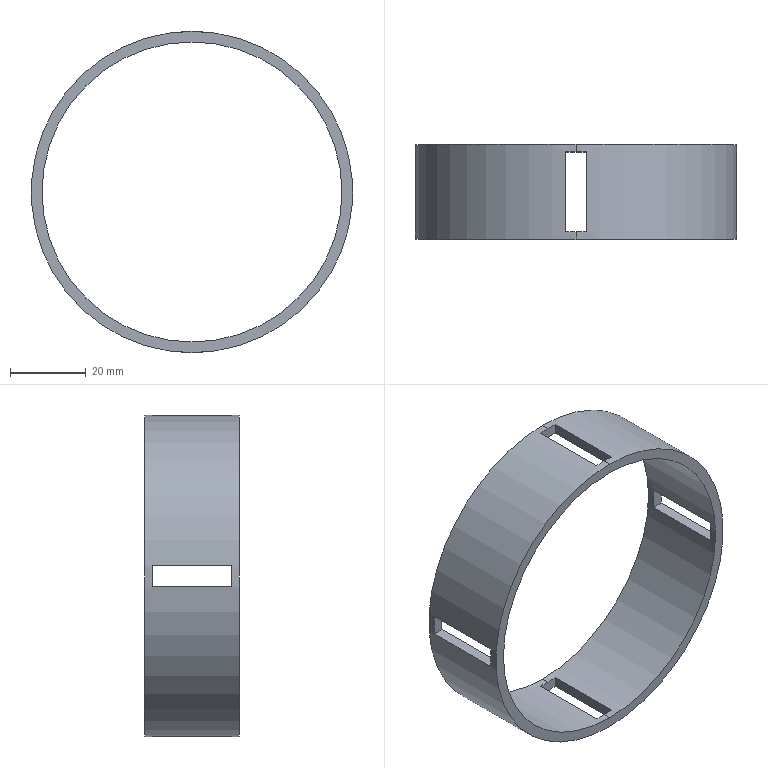Part | SolidWorks | features BaseBody 1 | 1 solid | 22 faces | box 84.688 x 25 x 84.688 mm | volume 16756 mm3 | plane 18 | cylinder 4 | commonest cylinder face diameters 79.062 x2 84.687 x2
STEP:
#1=CARTESIAN_POINT('',(-2132.95,780.069,-1538.093));
#2=VERTEX_POINT('',#1);
#3=CARTESIAN_POINT('',(-2132.95,780.069,-1617.156));
#4=VERTEX_POINT('',#3);
#5=CARTESIAN_POINT('',(-2132.95,780.069,-1577.624));
#6=DIRECTION('',(0.,1.,0.));
#7=DIRECTION('',(0.,0.,1.));
#8=AXIS2_PLACEMENT_3D('',#5,#6,#7);
#9=CIRCLE('',#8,39.531);
#10=EDGE_CURVE('',#2,#4,#9,.T.);
#11=ORIENTED_EDGE('',*,*,#10,.F.);
#12=CARTESIAN_POINT('',(-2132.95,780.069,-1577.624));
#13=DIRECTION('',(0.,1.,0.));
#14=DIRECTION('',(0.,0.,-1.));
#15=AXIS2_PLACEMENT_3D('',#12,#13,#14);
#16=CIRCLE('',#15,39.531);
#17=EDGE_CURVE('',#4,#2,#16,.T.);
#18=ORIENTED_EDGE('',*,*,#17,.F.);
#19=EDGE_LOOP('',(#11,#18));
#20=FACE_BOUND('',#19,.T.);
#21=CARTESIAN_POINT('',(-2132.95,780.069,-1619.968));
#22=VERTEX_POINT('',#21);
#23=CARTESIAN_POINT('',(-2132.95,780.069,-1535.281));
#24=VERTEX_POINT('',#23);
#25=CARTESIAN_POINT('',(-2132.95,780.069,-1577.624));
#26=DIRECTION('',(0.,1.,0.));
#27=DIRECTION('',(0.,0.,-1.));
#28=AXIS2_PLACEMENT_3D('',#25,#26,#27);
#29=CIRCLE('',#28,42.344);
#30=EDGE_CURVE('',#22,#24,#29,.T.);
#31=ORIENTED_EDGE('',*,*,#30,.T.);
#32=CARTESIAN_POINT('',(-2132.95,780.069,-1577.624));
#33=DIRECTION('',(0.,1.,0.));
#34=DIRECTION('',(0.,0.,1.));
#35=AXIS2_PLACEMENT_3D('',#32,#33,#34);
#36=CIRCLE('',#35,42.344);
#37=EDGE_CURVE('',#24,#22,#36,.T.);
#38=ORIENTED_EDGE('',*,*,#37,.T.);
#39=EDGE_LOOP('',(#31,#38));
#40=FACE_OUTER_BOUND('',#39,.T.);
#41=CARTESIAN_POINT('',(-2086.372,780.069,-1531.046));
#42=DIRECTION('',(0.,1.,0.));
#43=DIRECTION('',(1.,0.,0.));
#44=AXIS2_PLACEMENT_3D('',#41,#42,#43);
#45=PLANE('',#44);
#46=ADVANCED_FACE('',(#20,#40),#45,.T.);
#47=CARTESIAN_POINT('',(-2132.95,755.069,-1538.093));
#48=VERTEX_POINT('',#47);
#49=CARTESIAN_POINT('',(-2132.95,755.069,-1617.156));
#50=VERTEX_POINT('',#49);
#51=CARTESIAN_POINT('',(-2132.95,755.069,-1577.624));
#52=DIRECTION('',(0.,-1.,0.));
#53=DIRECTION('',(0.,0.,1.));
#54=AXIS2_PLACEMENT_3D('',#51,#52,#53);
#55=CIRCLE('',#54,39.531);
#56=EDGE_CURVE('',#48,#50,#55,.T.);
#57=ORIENTED_EDGE('',*,*,#56,.F.);
#58=CARTESIAN_POINT('',(-2132.95,755.069,-1577.624));
#59=DIRECTION('',(0.,-1.,0.));
#60=DIRECTION('',(0.,0.,-1.));
#61=AXIS2_PLACEMENT_3D('',#58,#59,#60);
#62=CIRCLE('',#61,39.531);
#63=EDGE_CURVE('',#50,#48,#62,.T.);
#64=ORIENTED_EDGE('',*,*,#63,.F.);
#65=EDGE_LOOP('',(#57,#64));
#66=FACE_BOUND('',#65,.T.);
#67=CARTESIAN_POINT('',(-2132.95,755.069,-1619.968));
#68=VERTEX_POINT('',#67);
#69=CARTESIAN_POINT('',(-2132.95,755.069,-1535.281));
#70=VERTEX_POINT('',#69);
#71=CARTESIAN_POINT('',(-2132.95,755.069,-1577.624));
#72=DIRECTION('',(0.,-1.,0.));
#73=DIRECTION('',(0.,0.,-1.));
#74=AXIS2_PLACEMENT_3D('',#71,#72,#73);
#75=CIRCLE('',#74,42.344);
#76=EDGE_CURVE('',#68,#70,#75,.T.);
#77=ORIENTED_EDGE('',*,*,#76,.T.);
#78=CARTESIAN_POINT('',(-2132.95,755.069,-1577.624));
#79=DIRECTION('',(0.,-1.,0.));
#80=DIRECTION('',(0.,0.,1.));
#81=AXIS2_PLACEMENT_3D('',#78,#79,#80);
#82=CIRCLE('',#81,42.344);
#83=EDGE_CURVE('',#70,#68,#82,.T.);
#84=ORIENTED_EDGE('',*,*,#83,.T.);
#85=EDGE_LOOP('',(#77,#84));
#86=FACE_OUTER_BOUND('',#85,.T.);
#87=CARTESIAN_POINT('',(-2086.372,755.069,-1624.203));
#88=DIRECTION('',(0.,-1.,0.));
#89=DIRECTION('',(0.,0.,-1.));
#90=AXIS2_PLACEMENT_3D('',#87,#88,#89);
#91=PLANE('',#90);
#92=ADVANCED_FACE('',(#66,#86),#91,.T.);
#93=CARTESIAN_POINT('',(-2090.699,757.069,-1574.812));
#94=VERTEX_POINT('',#93);
#95=CARTESIAN_POINT('',(-2090.699,757.069,-1580.437));
#96=VERTEX_POINT('',#95);
#97=CARTESIAN_POINT('',(-2132.95,757.069,-1577.624));
#98=DIRECTION('',(0.,1.,0.));
#99=DIRECTION('',(0.9978,0.,0.06642));
#100=AXIS2_PLACEMENT_3D('',#97,#98,#99);
#101=CIRCLE('',#100,42.344);
#102=EDGE_CURVE('',#94,#96,#101,.T.);
#103=ORIENTED_EDGE('',*,*,#102,.F.);
#104=CARTESIAN_POINT('',(-2090.699,778.069,-1574.812));
#105=VERTEX_POINT('',#104);
#106=CARTESIAN_POINT('',(-2090.699,757.069,-1574.812));
#107=DIRECTION('',(0.,1.,0.));
#108=VECTOR('',#107,1000.);
#109=LINE('',#106,#108);
#110=EDGE_CURVE('',#94,#105,#109,.T.);
#111=ORIENTED_EDGE('',*,*,#110,.T.);
#112=CARTESIAN_POINT('',(-2090.699,778.069,-1580.437));
#113=VERTEX_POINT('',#112);
#114=CARTESIAN_POINT('',(-2132.95,778.069,-1577.624));
#115=DIRECTION('',(0.,-1.,0.));
#116=DIRECTION('',(0.9978,0.,-0.06642));
#117=AXIS2_PLACEMENT_3D('',#114,#115,#116);
#118=CIRCLE('',#117,42.344);
#119=EDGE_CURVE('',#113,#105,#118,.T.);
#120=ORIENTED_EDGE('',*,*,#119,.F.);
#121=CARTESIAN_POINT('',(-2090.699,778.069,-1580.437));
#122=DIRECTION('',(0.,-1.,0.));
#123=VECTOR('',#122,1000.);
#124=LINE('',#121,#123);
#125=EDGE_CURVE('',#113,#96,#124,.T.);
#126=ORIENTED_EDGE('',*,*,#125,.T.);
#127=EDGE_LOOP('',(#103,#111,#120,#126));
#128=FACE_BOUND('',#127,.T.);
#129=CARTESIAN_POINT('',(-2132.95,757.069,-1619.968));
#130=VERTEX_POINT('',#129);
#131=CARTESIAN_POINT('',(-2132.95,755.069,-1619.968));
#132=DIRECTION('',(0.,1.,0.));
#133=VECTOR('',#132,1000.);
#134=LINE('',#131,#133);
#135=EDGE_CURVE('',#68,#130,#134,.T.);
#136=ORIENTED_EDGE('',*,*,#135,.T.);
#137=CARTESIAN_POINT('',(-2130.137,757.069,-1619.875));
#138=VERTEX_POINT('',#137);
#139=CARTESIAN_POINT('',(-2132.95,757.069,-1577.624));
#140=DIRECTION('',(0.,1.,0.));
#141=DIRECTION('',(0.06642,0.,-0.9978));
#142=AXIS2_PLACEMENT_3D('',#139,#140,#141);
#143=CIRCLE('',#142,42.344);
#144=EDGE_CURVE('',#138,#130,#143,.T.);
#145=ORIENTED_EDGE('',*,*,#144,.F.);
#146=CARTESIAN_POINT('',(-2130.137,778.069,-1619.875));
#147=VERTEX_POINT('',#146);
#148=CARTESIAN_POINT('',(-2130.137,757.069,-1619.875));
#149=DIRECTION('',(0.,1.,0.));
#150=VECTOR('',#149,1000.);
#151=LINE('',#148,#150);
#152=EDGE_CURVE('',#138,#147,#151,.T.);
#153=ORIENTED_EDGE('',*,*,#152,.T.);
#154=CARTESIAN_POINT('',(-2132.95,778.069,-1619.968));
#155=VERTEX_POINT('',#154);
#156=CARTESIAN_POINT('',(-2132.95,778.069,-1577.624));
#157=DIRECTION('',(0.,-1.,0.));
#158=DIRECTION('',(0.,0.,-1.));
#159=AXIS2_PLACEMENT_3D('',#156,#157,#158);
#160=CIRCLE('',#159,42.344);
#161=EDGE_CURVE('',#155,#147,#160,.T.);
#162=ORIENTED_EDGE('',*,*,#161,.F.);
#163=CARTESIAN_POINT('',(-2132.95,778.069,-1619.968));
#164=DIRECTION('',(0.,1.,0.));
#165=VECTOR('',#164,1000.);
#166=LINE('',#163,#165);
#167=EDGE_CURVE('',#155,#22,#166,.T.);
#168=ORIENTED_EDGE('',*,*,#167,.T.);
#169=ORIENTED_EDGE('',*,*,#37,.F.);
#170=CARTESIAN_POINT('',(-2132.95,778.069,-1535.281));
#171=VERTEX_POINT('',#170);
#172=CARTESIAN_POINT('',(-2132.95,780.069,-1535.281));
#173=DIRECTION('',(0.,-1.,0.));
#174=VECTOR('',#173,1000.);
#175=LINE('',#172,#174);
#176=EDGE_CURVE('',#24,#171,#175,.T.);
#177=ORIENTED_EDGE('',*,*,#176,.T.);
#178=CARTESIAN_POINT('',(-2130.137,778.069,-1535.374));
#179=VERTEX_POINT('',#178);
#180=CARTESIAN_POINT('',(-2132.95,778.069,-1577.624));
#181=DIRECTION('',(0.,-1.,0.));
#182=DIRECTION('',(0.06642,0.,0.9978));
#183=AXIS2_PLACEMENT_3D('',#180,#181,#182);
#184=CIRCLE('',#183,42.344);
#185=EDGE_CURVE('',#179,#171,#184,.T.);
#186=ORIENTED_EDGE('',*,*,#185,.F.);
#187=CARTESIAN_POINT('',(-2130.137,757.069,-1535.374));
#188=VERTEX_POINT('',#187);
#189=CARTESIAN_POINT('',(-2130.137,778.069,-1535.374));
#190=DIRECTION('',(0.,-1.,0.));
#191=VECTOR('',#190,1000.);
#192=LINE('',#189,#191);
#193=EDGE_CURVE('',#179,#188,#192,.T.);
#194=ORIENTED_EDGE('',*,*,#193,.T.);
#195=CARTESIAN_POINT('',(-2132.95,757.069,-1535.281));
#196=VERTEX_POINT('',#195);
#197=CARTESIAN_POINT('',(-2132.95,757.069,-1577.624));
#198=DIRECTION('',(0.,1.,0.));
#199=DIRECTION('',(0.,0.,1.));
#200=AXIS2_PLACEMENT_3D('',#197,#198,#199);
#201=CIRCLE('',#200,42.344);
#202=EDGE_CURVE('',#196,#188,#201,.T.);
#203=ORIENTED_EDGE('',*,*,#202,.F.);
#204=CARTESIAN_POINT('',(-2132.95,757.069,-1535.281));
#205=DIRECTION('',(0.,-1.,0.));
#206=VECTOR('',#205,1000.);
#207=LINE('',#204,#206);
#208=EDGE_CURVE('',#196,#70,#207,.T.);
#209=ORIENTED_EDGE('',*,*,#208,.T.);
#210=ORIENTED_EDGE('',*,*,#76,.F.);
#211=EDGE_LOOP('',(#136,#145,#153,#162,#168,#169,#177,#186,#194,#203,#209,#210));
#212=FACE_OUTER_BOUND('',#211,.T.);
#213=CARTESIAN_POINT('',(-2132.95,753.819,-1577.624));
#214=DIRECTION('',(0.,-1.,0.));
#215=DIRECTION('',(-0.08716,0.,-0.9962));
#216=AXIS2_PLACEMENT_3D('',#213,#214,#215);
#217=CYLINDRICAL_SURFACE('',#216,42.344);
#218=ADVANCED_FACE('',(#128,#212),#217,.T.);
#219=CARTESIAN_POINT('',(-2093.519,757.069,-1574.812));
#220=VERTEX_POINT('',#219);
#221=CARTESIAN_POINT('',(-2093.519,757.069,-1580.437));
#222=VERTEX_POINT('',#221);
#223=CARTESIAN_POINT('',(-2132.95,757.069,-1577.624));
#224=DIRECTION('',(0.,1.,0.));
#225=DIRECTION('',(0.9975,0.,0.07115));
#226=AXIS2_PLACEMENT_3D('',#223,#224,#225);
#227=CIRCLE('',#226,39.531);
#228=EDGE_CURVE('',#220,#222,#227,.T.);
#229=ORIENTED_EDGE('',*,*,#228,.T.);
#230=CARTESIAN_POINT('',(-2093.519,778.069,-1580.437));
#231=VERTEX_POINT('',#230);
#232=CARTESIAN_POINT('',(-2093.519,757.069,-1580.437));
#233=DIRECTION('',(0.,1.,0.));
#234=VECTOR('',#233,1000.);
#235=LINE('',#232,#234);
#236=EDGE_CURVE('',#222,#231,#235,.T.);
#237=ORIENTED_EDGE('',*,*,#236,.T.);
#238=CARTESIAN_POINT('',(-2093.519,778.069,-1574.812));
#239=VERTEX_POINT('',#238);
#240=CARTESIAN_POINT('',(-2132.95,778.069,-1577.624));
#241=DIRECTION('',(0.,-1.,0.));
#242=DIRECTION('',(0.9975,0.,-0.07115));
#243=AXIS2_PLACEMENT_3D('',#240,#241,#242);
#244=CIRCLE('',#243,39.531);
#245=EDGE_CURVE('',#231,#239,#244,.T.);
#246=ORIENTED_EDGE('',*,*,#245,.T.);
#247=CARTESIAN_POINT('',(-2093.519,778.069,-1574.812));
#248=DIRECTION('',(0.,-1.,0.));
#249=VECTOR('',#248,1000.);
#250=LINE('',#247,#249);
#251=EDGE_CURVE('',#239,#220,#250,.T.);
#252=ORIENTED_EDGE('',*,*,#251,.T.);
#253=EDGE_LOOP('',(#229,#237,#246,#252));
#254=FACE_BOUND('',#253,.T.);
#255=CARTESIAN_POINT('',(-2132.95,778.069,-1617.156));
#256=VERTEX_POINT('',#255);
#257=CARTESIAN_POINT('',(-2132.95,780.069,-1617.156));
#258=DIRECTION('',(0.,-1.,0.));
#259=VECTOR('',#258,1000.);
#260=LINE('',#257,#259);
#261=EDGE_CURVE('',#4,#256,#260,.T.);
#262=ORIENTED_EDGE('',*,*,#261,.T.);
#263=CARTESIAN_POINT('',(-2130.137,778.069,-1617.055));
#264=VERTEX_POINT('',#263);
#265=CARTESIAN_POINT('',(-2132.95,778.069,-1577.624));
#266=DIRECTION('',(0.,-1.,0.));
#267=DIRECTION('',(0.,0.,-1.));
#268=AXIS2_PLACEMENT_3D('',#265,#266,#267);
#269=CIRCLE('',#268,39.531);
#270=EDGE_CURVE('',#256,#264,#269,.T.);
#271=ORIENTED_EDGE('',*,*,#270,.T.);
#272=CARTESIAN_POINT('',(-2130.137,757.069,-1617.055));
#273=VERTEX_POINT('',#272);
#274=CARTESIAN_POINT('',(-2130.137,778.069,-1617.055));
#275=DIRECTION('',(0.,-1.,0.));
#276=VECTOR('',#275,1000.);
#277=LINE('',#274,#276);
#278=EDGE_CURVE('',#264,#273,#277,.T.);
#279=ORIENTED_EDGE('',*,*,#278,.T.);
#280=CARTESIAN_POINT('',(-2132.95,757.069,-1617.156));
#281=VERTEX_POINT('',#280);
#282=CARTESIAN_POINT('',(-2132.95,757.069,-1577.624));
#283=DIRECTION('',(0.,1.,0.));
#284=DIRECTION('',(0.07115,0.,-0.9975));
#285=AXIS2_PLACEMENT_3D('',#282,#283,#284);
#286=CIRCLE('',#285,39.531);
#287=EDGE_CURVE('',#273,#281,#286,.T.);
#288=ORIENTED_EDGE('',*,*,#287,.T.);
#289=CARTESIAN_POINT('',(-2132.95,757.069,-1617.156));
#290=DIRECTION('',(0.,-1.,0.));
#291=VECTOR('',#290,1000.);
#292=LINE('',#289,#291);
#293=EDGE_CURVE('',#281,#50,#292,.T.);
#294=ORIENTED_EDGE('',*,*,#293,.T.);
#295=ORIENTED_EDGE('',*,*,#63,.T.);
#296=CARTESIAN_POINT('',(-2132.95,757.069,-1538.093));
#297=VERTEX_POINT('',#296);
#298=CARTESIAN_POINT('',(-2132.95,755.069,-1538.093));
#299=DIRECTION('',(0.,1.,0.));
#300=VECTOR('',#299,1000.);
#301=LINE('',#298,#300);
#302=EDGE_CURVE('',#48,#297,#301,.T.);
#303=ORIENTED_EDGE('',*,*,#302,.T.);
#304=CARTESIAN_POINT('',(-2130.137,757.069,-1538.193));
#305=VERTEX_POINT('',#304);
#306=CARTESIAN_POINT('',(-2132.95,757.069,-1577.624));
#307=DIRECTION('',(0.,1.,0.));
#308=DIRECTION('',(0.,0.,1.));
#309=AXIS2_PLACEMENT_3D('',#306,#307,#308);
#310=CIRCLE('',#309,39.531);
#311=EDGE_CURVE('',#297,#305,#310,.T.);
#312=ORIENTED_EDGE('',*,*,#311,.T.);
#313=CARTESIAN_POINT('',(-2130.137,778.069,-1538.193));
#314=VERTEX_POINT('',#313);
#315=CARTESIAN_POINT('',(-2130.137,757.069,-1538.193));
#316=DIRECTION('',(0.,1.,0.));
#317=VECTOR('',#316,1000.);
#318=LINE('',#315,#317);
#319=EDGE_CURVE('',#305,#314,#318,.T.);
#320=ORIENTED_EDGE('',*,*,#319,.T.);
#321=CARTESIAN_POINT('',(-2132.95,778.069,-1538.093));
#322=VERTEX_POINT('',#321);
#323=CARTESIAN_POINT('',(-2132.95,778.069,-1577.624));
#324=DIRECTION('',(0.,-1.,0.));
#325=DIRECTION('',(0.07115,0.,0.9975));
#326=AXIS2_PLACEMENT_3D('',#323,#324,#325);
#327=CIRCLE('',#326,39.531);
#328=EDGE_CURVE('',#314,#322,#327,.T.);
#329=ORIENTED_EDGE('',*,*,#328,.T.);
#330=CARTESIAN_POINT('',(-2132.95,778.069,-1538.093));
#331=DIRECTION('',(0.,1.,0.));
#332=VECTOR('',#331,1000.);
#333=LINE('',#330,#332);
#334=EDGE_CURVE('',#322,#2,#333,.T.);
#335=ORIENTED_EDGE('',*,*,#334,.T.);
#336=ORIENTED_EDGE('',*,*,#10,.T.);
#337=EDGE_LOOP('',(#262,#271,#279,#288,#294,#295,#303,#312,#320,#329,#335,#336));
#338=FACE_OUTER_BOUND('',#337,.T.);
#339=CARTESIAN_POINT('',(-2132.95,781.319,-1577.624));
#340=DIRECTION('',(0.,-1.,0.));
#341=DIRECTION('',(-0.08716,0.,-0.9962));
#342=AXIS2_PLACEMENT_3D('',#339,#340,#341);
#343=CYLINDRICAL_SURFACE('',#342,39.531);
#344=ADVANCED_FACE('',(#254,#338),#343,.F.);
#345=CARTESIAN_POINT('',(-2135.762,757.069,-1617.055));
#346=VERTEX_POINT('',#345);
#347=CARTESIAN_POINT('',(-2135.762,778.069,-1617.055));
#348=VERTEX_POINT('',#347);
#349=CARTESIAN_POINT('',(-2135.762,757.069,-1617.055));
#350=DIRECTION('',(0.,1.,0.));
#351=VECTOR('',#350,1000.);
#352=LINE('',#349,#351);
#353=EDGE_CURVE('',#346,#348,#352,.T.);
#354=ORIENTED_EDGE('',*,*,#353,.F.);
#355=CARTESIAN_POINT('',(-2135.762,757.069,-1619.875));
#356=VERTEX_POINT('',#355);
#357=CARTESIAN_POINT('',(-2135.762,757.069,-1617.055));
#358=DIRECTION('',(0.,0.,-1.));
#359=VECTOR('',#358,1000.);
#360=LINE('',#357,#359);
#361=EDGE_CURVE('',#346,#356,#360,.T.);
#362=ORIENTED_EDGE('',*,*,#361,.T.);
#363=CARTESIAN_POINT('',(-2135.762,778.069,-1619.875));
#364=VERTEX_POINT('',#363);
#365=CARTESIAN_POINT('',(-2135.762,778.069,-1619.875));
#366=DIRECTION('',(0.,-1.,0.));
#367=VECTOR('',#366,1000.);
#368=LINE('',#365,#367);
#369=EDGE_CURVE('',#364,#356,#368,.T.);
#370=ORIENTED_EDGE('',*,*,#369,.F.);
#371=CARTESIAN_POINT('',(-2135.762,778.069,-1619.875));
#372=DIRECTION('',(0.,0.,1.));
#373=VECTOR('',#372,1000.);
#374=LINE('',#371,#373);
#375=EDGE_CURVE('',#364,#348,#374,.T.);
#376=ORIENTED_EDGE('',*,*,#375,.T.);
#377=EDGE_LOOP('',(#354,#362,#370,#376));
#378=FACE_OUTER_BOUND('',#377,.T.);
#379=CARTESIAN_POINT('',(-2135.762,779.119,-1616.005));
#380=DIRECTION('',(1.,0.,0.));
#381=DIRECTION('',(0.,1.,0.));
#382=AXIS2_PLACEMENT_3D('',#379,#380,#381);
#383=PLANE('',#382);
#384=ADVANCED_FACE('',(#378),#383,.T.);
#385=ORIENTED_EDGE('',*,*,#287,.F.);
#386=CARTESIAN_POINT('',(-2130.137,757.069,-1619.875));
#387=DIRECTION('',(0.,0.,1.));
#388=VECTOR('',#387,1000.);
#389=LINE('',#386,#388);
#390=EDGE_CURVE('',#138,#273,#389,.T.);
#391=ORIENTED_EDGE('',*,*,#390,.F.);
#392=ORIENTED_EDGE('',*,*,#144,.T.);
#393=CARTESIAN_POINT('',(-2132.95,757.069,-1577.624));
#394=DIRECTION('',(0.,1.,0.));
#395=DIRECTION('',(0.,0.,-1.));
#396=AXIS2_PLACEMENT_3D('',#393,#394,#395);
#397=CIRCLE('',#396,42.344);
#398=EDGE_CURVE('',#130,#356,#397,.T.);
#399=ORIENTED_EDGE('',*,*,#398,.T.);
#400=ORIENTED_EDGE('',*,*,#361,.F.);
#401=CARTESIAN_POINT('',(-2132.95,757.069,-1577.624));
#402=DIRECTION('',(0.,1.,0.));
#403=DIRECTION('',(0.,0.,-1.));
#404=AXIS2_PLACEMENT_3D('',#401,#402,#403);
#405=CIRCLE('',#404,39.531);
#406=EDGE_CURVE('',#281,#346,#405,.T.);
#407=ORIENTED_EDGE('',*,*,#406,.F.);
#408=EDGE_LOOP('',(#385,#391,#392,#399,#400,#407));
#409=FACE_OUTER_BOUND('',#408,.T.);
#410=CARTESIAN_POINT('',(-2129.856,757.069,-1616.774));
#411=DIRECTION('',(0.,1.,0.));
#412=DIRECTION('',(1.,0.,0.));
#413=AXIS2_PLACEMENT_3D('',#410,#411,#412);
#414=PLANE('',#413);
#415=ADVANCED_FACE('',(#409),#414,.T.);
#416=ORIENTED_EDGE('',*,*,#278,.F.);
#417=CARTESIAN_POINT('',(-2130.137,778.069,-1617.055));
#418=DIRECTION('',(0.,0.,-1.));
#419=VECTOR('',#418,1000.);
#420=LINE('',#417,#419);
#421=EDGE_CURVE('',#264,#147,#420,.T.);
#422=ORIENTED_EDGE('',*,*,#421,.T.);
#423=ORIENTED_EDGE('',*,*,#152,.F.);
#424=ORIENTED_EDGE('',*,*,#390,.T.);
#425=EDGE_LOOP('',(#416,#422,#423,#424));
#426=FACE_OUTER_BOUND('',#425,.T.);
#427=CARTESIAN_POINT('',(-2130.137,756.019,-1616.005));
#428=DIRECTION('',(-1.,0.,0.));
#429=DIRECTION('',(0.,0.,1.));
#430=AXIS2_PLACEMENT_3D('',#427,#428,#429);
#431=PLANE('',#430);
#432=ADVANCED_FACE('',(#426),#431,.T.);
#433=CARTESIAN_POINT('',(-2132.95,778.069,-1577.624));
#434=DIRECTION('',(0.,-1.,0.));
#435=DIRECTION('',(-0.07115,0.,-0.9975));
#436=AXIS2_PLACEMENT_3D('',#433,#434,#435);
#437=CIRCLE('',#436,39.531);
#438=EDGE_CURVE('',#348,#256,#437,.T.);
#439=ORIENTED_EDGE('',*,*,#438,.F.);
#440=ORIENTED_EDGE('',*,*,#375,.F.);
#441=CARTESIAN_POINT('',(-2132.95,778.069,-1577.624));
#442=DIRECTION('',(0.,-1.,0.));
#443=DIRECTION('',(-0.06642,0.,-0.9978));
#444=AXIS2_PLACEMENT_3D('',#441,#442,#443);
#445=CIRCLE('',#444,42.344);
#446=EDGE_CURVE('',#364,#155,#445,.T.);
#447=ORIENTED_EDGE('',*,*,#446,.T.);
#448=ORIENTED_EDGE('',*,*,#161,.T.);
#449=ORIENTED_EDGE('',*,*,#421,.F.);
#450=ORIENTED_EDGE('',*,*,#270,.F.);
#451=EDGE_LOOP('',(#439,#440,#447,#448,#449,#450));
#452=FACE_OUTER_BOUND('',#451,.T.);
#453=CARTESIAN_POINT('',(-2136.043,778.069,-1616.774));
#454=DIRECTION('',(0.,-1.,0.));
#455=DIRECTION('',(0.,0.,-1.));
#456=AXIS2_PLACEMENT_3D('',#453,#454,#455);
#457=PLANE('',#456);
#458=ADVANCED_FACE('',(#452),#457,.T.);
#459=CARTESIAN_POINT('',(-2172.381,757.069,-1574.812));
#460=VERTEX_POINT('',#459);
#461=CARTESIAN_POINT('',(-2172.381,778.069,-1574.812));
#462=VERTEX_POINT('',#461);
#463=CARTESIAN_POINT('',(-2172.381,757.069,-1574.812));
#464=DIRECTION('',(0.,1.,0.));
#465=VECTOR('',#464,1000.);
#466=LINE('',#463,#465);
#467=EDGE_CURVE('',#460,#462,#466,.T.);
#468=ORIENTED_EDGE('',*,*,#467,.F.);
#469=CARTESIAN_POINT('',(-2175.2,757.069,-1574.812));
#470=VERTEX_POINT('',#469);
#471=CARTESIAN_POINT('',(-2172.381,757.069,-1574.812));
#472=DIRECTION('',(-1.,0.,0.));
#473=VECTOR('',#472,1000.);
#474=LINE('',#471,#473);
#475=EDGE_CURVE('',#460,#470,#474,.T.);
#476=ORIENTED_EDGE('',*,*,#475,.T.);
#477=CARTESIAN_POINT('',(-2175.2,778.069,-1574.812));
#478=VERTEX_POINT('',#477);
#479=CARTESIAN_POINT('',(-2175.2,778.069,-1574.812));
#480=DIRECTION('',(0.,-1.,0.));
#481=VECTOR('',#480,1000.);
#482=LINE('',#479,#481);
#483=EDGE_CURVE('',#478,#470,#482,.T.);
#484=ORIENTED_EDGE('',*,*,#483,.F.);
#485=CARTESIAN_POINT('',(-2175.2,778.069,-1574.812));
#486=DIRECTION('',(1.,0.,0.));
#487=VECTOR('',#486,1000.);
#488=LINE('',#485,#487);
#489=EDGE_CURVE('',#478,#462,#488,.T.);
#490=ORIENTED_EDGE('',*,*,#489,.T.);
#491=EDGE_LOOP('',(#468,#476,#484,#490));
#492=FACE_OUTER_BOUND('',#491,.T.);
#493=CARTESIAN_POINT('',(-2171.331,779.119,-1574.812));
#494=DIRECTION('',(0.,0.,-1.));
#495=DIRECTION('',(0.,-1.,0.));
#496=AXIS2_PLACEMENT_3D('',#493,#494,#495);
#497=PLANE('',#496);
#498=ADVANCED_FACE('',(#492),#497,.T.);
#499=CARTESIAN_POINT('',(-2172.381,757.069,-1580.437));
#500=VERTEX_POINT('',#499);
#501=CARTESIAN_POINT('',(-2132.95,757.069,-1577.624));
#502=DIRECTION('',(0.,1.,0.));
#503=DIRECTION('',(-0.9975,0.,-0.07115));
#504=AXIS2_PLACEMENT_3D('',#501,#502,#503);
#505=CIRCLE('',#504,39.531);
#506=EDGE_CURVE('',#500,#460,#505,.T.);
#507=ORIENTED_EDGE('',*,*,#506,.F.);
#508=CARTESIAN_POINT('',(-2175.2,757.069,-1580.437));
#509=VERTEX_POINT('',#508);
#510=CARTESIAN_POINT('',(-2175.2,757.069,-1580.437));
#511=DIRECTION('',(1.,0.,0.));
#512=VECTOR('',#511,1000.);
#513=LINE('',#510,#512);
#514=EDGE_CURVE('',#509,#500,#513,.T.);
#515=ORIENTED_EDGE('',*,*,#514,.F.);
#516=CARTESIAN_POINT('',(-2132.95,757.069,-1577.624));
#517=DIRECTION('',(0.,1.,0.));
#518=DIRECTION('',(-0.9978,0.,-0.06642));
#519=AXIS2_PLACEMENT_3D('',#516,#517,#518);
#520=CIRCLE('',#519,42.344);
#521=EDGE_CURVE('',#509,#470,#520,.T.);
#522=ORIENTED_EDGE('',*,*,#521,.T.);
#523=ORIENTED_EDGE('',*,*,#475,.F.);
#524=EDGE_LOOP('',(#507,#515,#522,#523));
#525=FACE_OUTER_BOUND('',#524,.T.);
#526=CARTESIAN_POINT('',(-2172.1,757.069,-1580.718));
#527=DIRECTION('',(0.,1.,0.));
#528=DIRECTION('',(1.,0.,0.));
#529=AXIS2_PLACEMENT_3D('',#526,#527,#528);
#530=PLANE('',#529);
#531=ADVANCED_FACE('',(#525),#530,.T.);
#532=CARTESIAN_POINT('',(-2172.381,778.069,-1580.437));
#533=VERTEX_POINT('',#532);
#534=CARTESIAN_POINT('',(-2172.381,778.069,-1580.437));
#535=DIRECTION('',(0.,-1.,0.));
#536=VECTOR('',#535,1000.);
#537=LINE('',#534,#536);
#538=EDGE_CURVE('',#533,#500,#537,.T.);
#539=ORIENTED_EDGE('',*,*,#538,.F.);
#540=CARTESIAN_POINT('',(-2175.2,778.069,-1580.437));
#541=VERTEX_POINT('',#540);
#542=CARTESIAN_POINT('',(-2172.381,778.069,-1580.437));
#543=DIRECTION('',(-1.,0.,0.));
#544=VECTOR('',#543,1000.);
#545=LINE('',#542,#544);
#546=EDGE_CURVE('',#533,#541,#545,.T.);
#547=ORIENTED_EDGE('',*,*,#546,.T.);
#548=CARTESIAN_POINT('',(-2175.2,757.069,-1580.437));
#549=DIRECTION('',(0.,1.,0.));
#550=VECTOR('',#549,1000.);
#551=LINE('',#548,#550);
#552=EDGE_CURVE('',#509,#541,#551,.T.);
#553=ORIENTED_EDGE('',*,*,#552,.F.);
#554=ORIENTED_EDGE('',*,*,#514,.T.);
#555=EDGE_LOOP('',(#539,#547,#553,#554));
#556=FACE_OUTER_BOUND('',#555,.T.);
#557=CARTESIAN_POINT('',(-2171.331,756.019,-1580.437));
#558=DIRECTION('',(0.,0.,1.));
#559=DIRECTION('',(1.,0.,0.));
#560=AXIS2_PLACEMENT_3D('',#557,#558,#559);
#561=PLANE('',#560);
#562=ADVANCED_FACE('',(#556),#561,.T.);
#563=CARTESIAN_POINT('',(-2132.95,778.069,-1577.624));
#564=DIRECTION('',(0.,-1.,0.));
#565=DIRECTION('',(-0.9975,0.,0.07115));
#566=AXIS2_PLACEMENT_3D('',#563,#564,#565);
#567=CIRCLE('',#566,39.531);
#568=EDGE_CURVE('',#462,#533,#567,.T.);
#569=ORIENTED_EDGE('',*,*,#568,.F.);
#570=ORIENTED_EDGE('',*,*,#489,.F.);
#571=CARTESIAN_POINT('',(-2132.95,778.069,-1577.624));
#572=DIRECTION('',(0.,-1.,0.));
#573=DIRECTION('',(-0.9978,0.,0.06642));
#574=AXIS2_PLACEMENT_3D('',#571,#572,#573);
#575=CIRCLE('',#574,42.344);
#576=EDGE_CURVE('',#478,#541,#575,.T.);
#577=ORIENTED_EDGE('',*,*,#576,.T.);
#578=ORIENTED_EDGE('',*,*,#546,.F.);
#579=EDGE_LOOP('',(#569,#570,#577,#578));
#580=FACE_OUTER_BOUND('',#579,.T.);
#581=CARTESIAN_POINT('',(-2172.1,778.069,-1574.531));
#582=DIRECTION('',(0.,-1.,0.));
#583=DIRECTION('',(0.,0.,-1.));
#584=AXIS2_PLACEMENT_3D('',#581,#582,#583);
#585=PLANE('',#584);
#586=ADVANCED_FACE('',(#580),#585,.T.);
#587=ORIENTED_EDGE('',*,*,#319,.F.);
#588=CARTESIAN_POINT('',(-2130.137,757.069,-1538.193));
#589=DIRECTION('',(0.,0.,1.));
#590=VECTOR('',#589,1000.);
#591=LINE('',#588,#590);
#592=EDGE_CURVE('',#305,#188,#591,.T.);
#593=ORIENTED_EDGE('',*,*,#592,.T.);
#594=ORIENTED_EDGE('',*,*,#193,.F.);
#595=CARTESIAN_POINT('',(-2130.137,778.069,-1535.374));
#596=DIRECTION('',(0.,0.,-1.));
#597=VECTOR('',#596,1000.);
#598=LINE('',#595,#597);
#599=EDGE_CURVE('',#179,#314,#598,.T.);
#600=ORIENTED_EDGE('',*,*,#599,.T.);
#601=EDGE_LOOP('',(#587,#593,#594,#600));
#602=FACE_OUTER_BOUND('',#601,.T.);
#603=CARTESIAN_POINT('',(-2130.137,779.119,-1539.243));
#604=DIRECTION('',(-1.,0.,0.));
#605=DIRECTION('',(0.,0.,1.));
#606=AXIS2_PLACEMENT_3D('',#603,#604,#605);
#607=PLANE('',#606);
#608=ADVANCED_FACE('',(#602),#607,.T.);
#609=CARTESIAN_POINT('',(-2135.762,757.069,-1538.193));
#610=VERTEX_POINT('',#609);
#611=CARTESIAN_POINT('',(-2132.95,757.069,-1577.624));
#612=DIRECTION('',(0.,1.,0.));
#613=DIRECTION('',(-0.07115,0.,0.9975));
#614=AXIS2_PLACEMENT_3D('',#611,#612,#613);
#615=CIRCLE('',#614,39.531);
#616=EDGE_CURVE('',#610,#297,#615,.T.);
#617=ORIENTED_EDGE('',*,*,#616,.F.);
#618=CARTESIAN_POINT('',(-2135.762,757.069,-1535.374));
#619=VERTEX_POINT('',#618);
#620=CARTESIAN_POINT('',(-2135.762,757.069,-1535.374));
#621=DIRECTION('',(0.,0.,-1.));
#622=VECTOR('',#621,1000.);
#623=LINE('',#620,#622);
#624=EDGE_CURVE('',#619,#610,#623,.T.);
#625=ORIENTED_EDGE('',*,*,#624,.F.);
#626=CARTESIAN_POINT('',(-2132.95,757.069,-1577.624));
#627=DIRECTION('',(0.,1.,0.));
#628=DIRECTION('',(-0.06642,0.,0.9978));
#629=AXIS2_PLACEMENT_3D('',#626,#627,#628);
#630=CIRCLE('',#629,42.344);
#631=EDGE_CURVE('',#619,#196,#630,.T.);
#632=ORIENTED_EDGE('',*,*,#631,.T.);
#633=ORIENTED_EDGE('',*,*,#202,.T.);
#634=ORIENTED_EDGE('',*,*,#592,.F.);
#635=ORIENTED_EDGE('',*,*,#311,.F.);
#636=EDGE_LOOP('',(#617,#625,#632,#633,#634,#635));
#637=FACE_OUTER_BOUND('',#636,.T.);
#638=CARTESIAN_POINT('',(-2136.043,757.069,-1538.475));
#639=DIRECTION('',(0.,1.,0.));
#640=DIRECTION('',(1.,0.,0.));
#641=AXIS2_PLACEMENT_3D('',#638,#639,#640);
#642=PLANE('',#641);
#643=ADVANCED_FACE('',(#637),#642,.T.);
#644=CARTESIAN_POINT('',(-2135.762,778.069,-1538.193));
#645=VERTEX_POINT('',#644);
#646=CARTESIAN_POINT('',(-2135.762,778.069,-1538.193));
#647=DIRECTION('',(0.,-1.,0.));
#648=VECTOR('',#647,1000.);
#649=LINE('',#646,#648);
#650=EDGE_CURVE('',#645,#610,#649,.T.);
#651=ORIENTED_EDGE('',*,*,#650,.F.);
#652=CARTESIAN_POINT('',(-2135.762,778.069,-1535.374));
#653=VERTEX_POINT('',#652);
#654=CARTESIAN_POINT('',(-2135.762,778.069,-1538.193));
#655=DIRECTION('',(0.,0.,1.));
#656=VECTOR('',#655,1000.);
#657=LINE('',#654,#656);
#658=EDGE_CURVE('',#645,#653,#657,.T.);
#659=ORIENTED_EDGE('',*,*,#658,.T.);
#660=CARTESIAN_POINT('',(-2135.762,757.069,-1535.374));
#661=DIRECTION('',(0.,1.,0.));
#662=VECTOR('',#661,1000.);
#663=LINE('',#660,#662);
#664=EDGE_CURVE('',#619,#653,#663,.T.);
#665=ORIENTED_EDGE('',*,*,#664,.F.);
#666=ORIENTED_EDGE('',*,*,#624,.T.);
#667=EDGE_LOOP('',(#651,#659,#665,#666));
#668=FACE_OUTER_BOUND('',#667,.T.);
#669=CARTESIAN_POINT('',(-2135.762,756.019,-1539.243));
#670=DIRECTION('',(1.,0.,0.));
#671=DIRECTION('',(0.,1.,0.));
#672=AXIS2_PLACEMENT_3D('',#669,#670,#671);
#673=PLANE('',#672);
#674=ADVANCED_FACE('',(#668),#673,.T.);
#675=ORIENTED_EDGE('',*,*,#328,.F.);
#676=ORIENTED_EDGE('',*,*,#599,.F.);
#677=ORIENTED_EDGE('',*,*,#185,.T.);
#678=CARTESIAN_POINT('',(-2132.95,778.069,-1577.624));
#679=DIRECTION('',(0.,-1.,0.));
#680=DIRECTION('',(0.,0.,1.));
#681=AXIS2_PLACEMENT_3D('',#678,#679,#680);
#682=CIRCLE('',#681,42.344);
#683=EDGE_CURVE('',#171,#653,#682,.T.);
#684=ORIENTED_EDGE('',*,*,#683,.T.);
#685=ORIENTED_EDGE('',*,*,#658,.F.);
#686=CARTESIAN_POINT('',(-2132.95,778.069,-1577.624));
#687=DIRECTION('',(0.,-1.,0.));
#688=DIRECTION('',(0.,0.,1.));
#689=AXIS2_PLACEMENT_3D('',#686,#687,#688);
#690=CIRCLE('',#689,39.531);
#691=EDGE_CURVE('',#322,#645,#690,.T.);
#692=ORIENTED_EDGE('',*,*,#691,.F.);
#693=EDGE_LOOP('',(#675,#676,#677,#684,#685,#692));
#694=FACE_OUTER_BOUND('',#693,.T.);
#695=CARTESIAN_POINT('',(-2129.856,778.069,-1538.475));
#696=DIRECTION('',(0.,-1.,0.));
#697=DIRECTION('',(0.,0.,-1.));
#698=AXIS2_PLACEMENT_3D('',#695,#696,#697);
#699=PLANE('',#698);
#700=ADVANCED_FACE('',(#694),#699,.T.);
#701=ORIENTED_EDGE('',*,*,#236,.F.);
#702=CARTESIAN_POINT('',(-2093.519,757.069,-1580.437));
#703=DIRECTION('',(1.,0.,0.));
#704=VECTOR('',#703,1000.);
#705=LINE('',#702,#704);
#706=EDGE_CURVE('',#222,#96,#705,.T.);
#707=ORIENTED_EDGE('',*,*,#706,.T.);
#708=ORIENTED_EDGE('',*,*,#125,.F.);
#709=CARTESIAN_POINT('',(-2090.699,778.069,-1580.437));
#710=DIRECTION('',(-1.,0.,0.));
#711=VECTOR('',#710,1000.);
#712=LINE('',#709,#711);
#713=EDGE_CURVE('',#113,#231,#712,.T.);
#714=ORIENTED_EDGE('',*,*,#713,.T.);
#715=EDGE_LOOP('',(#701,#707,#708,#714));
#716=FACE_OUTER_BOUND('',#715,.T.);
#717=CARTESIAN_POINT('',(-2094.569,779.119,-1580.437));
#718=DIRECTION('',(0.,0.,1.));
#719=DIRECTION('',(1.,0.,0.));
#720=AXIS2_PLACEMENT_3D('',#717,#718,#719);
#721=PLANE('',#720);
#722=ADVANCED_FACE('',(#716),#721,.T.);
#723=ORIENTED_EDGE('',*,*,#228,.F.);
#724=CARTESIAN_POINT('',(-2090.699,757.069,-1574.812));
#725=DIRECTION('',(-1.,0.,0.));
#726=VECTOR('',#725,1000.);
#727=LINE('',#724,#726);
#728=EDGE_CURVE('',#94,#220,#727,.T.);
#729=ORIENTED_EDGE('',*,*,#728,.F.);
#730=ORIENTED_EDGE('',*,*,#102,.T.);
#731=ORIENTED_EDGE('',*,*,#706,.F.);
#732=EDGE_LOOP('',(#723,#729,#730,#731));
#733=FACE_OUTER_BOUND('',#732,.T.);
#734=CARTESIAN_POINT('',(-2093.8,757.069,-1574.531));
#735=DIRECTION('',(0.,1.,0.));
#736=DIRECTION('',(1.,0.,0.));
#737=AXIS2_PLACEMENT_3D('',#734,#735,#736);
#738=PLANE('',#737);
#739=ADVANCED_FACE('',(#733),#738,.T.);
#740=ORIENTED_EDGE('',*,*,#251,.F.);
#741=CARTESIAN_POINT('',(-2093.519,778.069,-1574.812));
#742=DIRECTION('',(1.,0.,0.));
#743=VECTOR('',#742,1000.);
#744=LINE('',#741,#743);
#745=EDGE_CURVE('',#239,#105,#744,.T.);
#746=ORIENTED_EDGE('',*,*,#745,.T.);
#747=ORIENTED_EDGE('',*,*,#110,.F.);
#748=ORIENTED_EDGE('',*,*,#728,.T.);
#749=EDGE_LOOP('',(#740,#746,#747,#748));
#750=FACE_OUTER_BOUND('',#749,.T.);
#751=CARTESIAN_POINT('',(-2094.569,756.019,-1574.812));
#752=DIRECTION('',(0.,0.,-1.));
#753=DIRECTION('',(0.,-1.,0.));
#754=AXIS2_PLACEMENT_3D('',#751,#752,#753);
#755=PLANE('',#754);
#756=ADVANCED_FACE('',(#750),#755,.T.);
#757=ORIENTED_EDGE('',*,*,#245,.F.);
#758=ORIENTED_EDGE('',*,*,#713,.F.);
#759=ORIENTED_EDGE('',*,*,#119,.T.);
#760=ORIENTED_EDGE('',*,*,#745,.F.);
#761=EDGE_LOOP('',(#757,#758,#759,#760));
#762=FACE_OUTER_BOUND('',#761,.T.);
#763=CARTESIAN_POINT('',(-2093.8,778.069,-1580.718));
#764=DIRECTION('',(0.,-1.,0.));
#765=DIRECTION('',(0.,0.,-1.));
#766=AXIS2_PLACEMENT_3D('',#763,#764,#765);
#767=PLANE('',#766);
#768=ADVANCED_FACE('',(#762),#767,.T.);
#769=ORIENTED_EDGE('',*,*,#506,.T.);
#770=ORIENTED_EDGE('',*,*,#467,.T.);
#771=ORIENTED_EDGE('',*,*,#568,.T.);
#772=ORIENTED_EDGE('',*,*,#538,.T.);
#773=EDGE_LOOP('',(#769,#770,#771,#772));
#774=FACE_BOUND('',#773,.T.);
#775=ORIENTED_EDGE('',*,*,#261,.F.);
#776=ORIENTED_EDGE('',*,*,#17,.T.);
#777=ORIENTED_EDGE('',*,*,#334,.F.);
#778=ORIENTED_EDGE('',*,*,#691,.T.);
#779=ORIENTED_EDGE('',*,*,#650,.T.);
#780=ORIENTED_EDGE('',*,*,#616,.T.);
#781=ORIENTED_EDGE('',*,*,#302,.F.);
#782=ORIENTED_EDGE('',*,*,#56,.T.);
#783=ORIENTED_EDGE('',*,*,#293,.F.);
#784=ORIENTED_EDGE('',*,*,#406,.T.);
#785=ORIENTED_EDGE('',*,*,#353,.T.);
#786=ORIENTED_EDGE('',*,*,#438,.T.);
#787=EDGE_LOOP('',(#775,#776,#777,#778,#779,#780,#781,#782,#783,#784,#785,#786));
#788=FACE_OUTER_BOUND('',#787,.T.);
#789=CARTESIAN_POINT('',(-2132.95,781.319,-1577.624));
#790=DIRECTION('',(0.,-1.,0.));
#791=DIRECTION('',(0.08716,0.,0.9962));
#792=AXIS2_PLACEMENT_3D('',#789,#790,#791);
#793=CYLINDRICAL_SURFACE('',#792,39.531);
#794=ADVANCED_FACE('',(#774,#788),#793,.F.);
#795=ORIENTED_EDGE('',*,*,#521,.F.);
#796=ORIENTED_EDGE('',*,*,#552,.T.);
#797=ORIENTED_EDGE('',*,*,#576,.F.);
#798=ORIENTED_EDGE('',*,*,#483,.T.);
#799=EDGE_LOOP('',(#795,#796,#797,#798));
#800=FACE_BOUND('',#799,.T.);
#801=ORIENTED_EDGE('',*,*,#135,.F.);
#802=ORIENTED_EDGE('',*,*,#83,.F.);
#803=ORIENTED_EDGE('',*,*,#208,.F.);
#804=ORIENTED_EDGE('',*,*,#631,.F.);
#805=ORIENTED_EDGE('',*,*,#664,.T.);
#806=ORIENTED_EDGE('',*,*,#683,.F.);
#807=ORIENTED_EDGE('',*,*,#176,.F.);
#808=ORIENTED_EDGE('',*,*,#30,.F.);
#809=ORIENTED_EDGE('',*,*,#167,.F.);
#810=ORIENTED_EDGE('',*,*,#446,.F.);
#811=ORIENTED_EDGE('',*,*,#369,.T.);
#812=ORIENTED_EDGE('',*,*,#398,.F.);
#813=EDGE_LOOP('',(#801,#802,#803,#804,#805,#806,#807,#808,#809,#810,#811,#812));
#814=FACE_OUTER_BOUND('',#813,.T.);
#815=CARTESIAN_POINT('',(-2132.95,753.819,-1577.624));
#816=DIRECTION('',(0.,-1.,0.));
#817=DIRECTION('',(0.08716,0.,0.9962));
#818=AXIS2_PLACEMENT_3D('',#815,#816,#817);
#819=CYLINDRICAL_SURFACE('',#818,42.344);
#820=ADVANCED_FACE('',(#800,#814),#819,.T.);
#821=CLOSED_SHELL('',(#46,#92,#218,#344,#384,#415,#432,#458,#498,#531,#562,#586,#608,#643,#674,#700,#722,#739,#756,#768,#794,#820));
#822=MANIFOLD_SOLID_BREP('',#821);
#823=CARTESIAN_POINT('',(0.,0.,0.));
#824=DIRECTION('',(0.,0.,1.));
#825=DIRECTION('',(1.,0.,0.));
#826=AXIS2_PLACEMENT_3D('',#823,#824,#825);
#827=(LENGTH_UNIT()NAMED_UNIT(*)SI_UNIT(.MILLI.,.METRE.));
#828=UNCERTAINTY_MEASURE_WITH_UNIT(LENGTH_MEASURE(0.00001),#827,'','');
#829=(NAMED_UNIT(*)PLANE_ANGLE_UNIT()SI_UNIT($,.RADIAN.));
#830=(NAMED_UNIT(*)SI_UNIT($,.STERADIAN.)SOLID_ANGLE_UNIT());
#831=(GEOMETRIC_REPRESENTATION_CONTEXT(3)GLOBAL_UNCERTAINTY_ASSIGNED_CONTEXT((#828))GLOBAL_UNIT_ASSIGNED_CONTEXT((#827,#829,#830))REPRESENTATION_CONTEXT('',''));
#832=ADVANCED_BREP_SHAPE_REPRESENTATION('',(#822,#826),#831);